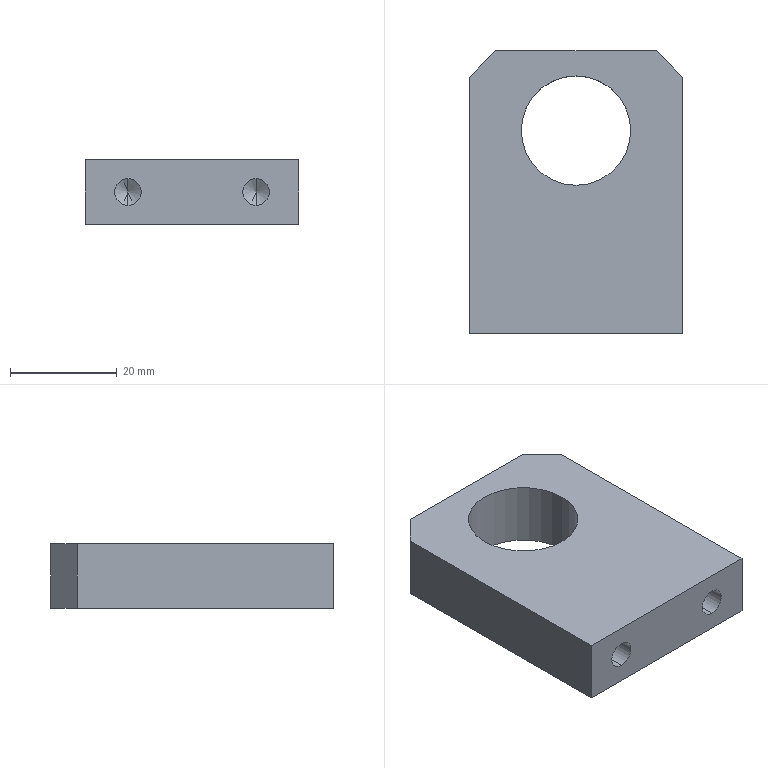Part | STEP file | 1 solid | 18 faces | box 40 x 53 x 12 mm | volume 20571 mm3 | plane 8 | cylinder 6 | cone 4 | commonest cylinder face diameters 5 x4 20.5 x2
STEP:
#1=CARTESIAN_POINT('',(0.,0.,0.));
#2=DIRECTION('',(0.,0.,1.));
#3=DIRECTION('',(1.,0.,0.));
#4=AXIS2_PLACEMENT_3D('',#1,#2,#3);
#5=CARTESIAN_POINT('',(8.,15.,3.5));
#6=VERTEX_POINT('',#5);
#7=CARTESIAN_POINT('',(8.,0.,3.5));
#8=VERTEX_POINT('',#7);
#9=CARTESIAN_POINT('',(8.,0.,3.5));
#10=DIRECTION('',(0.,-1.,0.));
#11=VECTOR('',#10,1.);
#12=LINE('',#9,#11);
#13=CARTESIAN_POINT('',(8.,0.,6.));
#14=DIRECTION('',(0.,-1.,0.));
#15=DIRECTION('',(0.,0.,-1.));
#16=AXIS2_PLACEMENT_3D('',#13,#14,#15);
#17=CYLINDRICAL_SURFACE('',#16,2.5);
#18=CARTESIAN_POINT('',(6.283,0.));
#19=DIRECTION('',(0.,1.));
#20=VECTOR('',#19,1.);
#21=LINE('',#18,#20);
#22=(GEOMETRIC_REPRESENTATION_CONTEXT(2)PARAMETRIC_REPRESENTATION_CONTEXT()REPRESENTATION_CONTEXT('',''));
#23=DEFINITIONAL_REPRESENTATION('',(#21),#22);
#24=PCURVE('',#17,#23);
#25=CARTESIAN_POINT('',(8.,0.,6.));
#26=DIRECTION('',(0.,-1.,0.));
#27=DIRECTION('',(0.,0.,-1.));
#28=AXIS2_PLACEMENT_3D('',#25,#26,#27);
#29=CYLINDRICAL_SURFACE('',#28,2.5);
#30=CARTESIAN_POINT('',(0.,0.));
#31=DIRECTION('',(0.,1.));
#32=VECTOR('',#31,1.);
#33=LINE('',#30,#32);
#34=(GEOMETRIC_REPRESENTATION_CONTEXT(2)PARAMETRIC_REPRESENTATION_CONTEXT()REPRESENTATION_CONTEXT('',''));
#35=DEFINITIONAL_REPRESENTATION('',(#33),#34);
#36=PCURVE('',#29,#35);
#37=SURFACE_CURVE('',#12,(#24,#36),.PCURVE_S1.);
#38=EDGE_CURVE('',#6,#8,#37,.T.);
#39=ORIENTED_EDGE('',*,*,#38,.T.);
#40=CARTESIAN_POINT('',(8.,0.,8.5));
#41=VERTEX_POINT('',#40);
#42=CARTESIAN_POINT('',(8.,0.,6.));
#43=DIRECTION('',(0.,-1.,0.));
#44=DIRECTION('',(0.,0.,-1.));
#45=AXIS2_PLACEMENT_3D('',#42,#43,#44);
#46=CIRCLE('',#45,2.5);
#47=CARTESIAN_POINT('',(0.,0.));
#48=DIRECTION('',(1.,0.));
#49=VECTOR('',#48,1.);
#50=LINE('',#47,#49);
#51=(GEOMETRIC_REPRESENTATION_CONTEXT(2)PARAMETRIC_REPRESENTATION_CONTEXT()REPRESENTATION_CONTEXT('',''));
#52=DEFINITIONAL_REPRESENTATION('',(#50),#51);
#53=PCURVE('',#17,#52);
#54=CARTESIAN_POINT('',(0.,0.,12.));
#55=DIRECTION('',(0.,1.,0.));
#56=DIRECTION('',(0.,0.,1.));
#57=AXIS2_PLACEMENT_3D('',#54,#55,#56);
#58=PLANE('',#57);
#59=CARTESIAN_POINT('',(-8.5,8.));
#60=CARTESIAN_POINT('',(-8.5,12.33));
#61=CARTESIAN_POINT('',(-4.75,10.165));
#62=CARTESIAN_POINT('',(-1.,8.));
#63=CARTESIAN_POINT('',(-4.75,5.835));
#64=CARTESIAN_POINT('',(-8.5,3.67));
#65=CARTESIAN_POINT('',(-8.5,8.));
#66=(BOUNDED_CURVE()B_SPLINE_CURVE(2,(#59,#60,#61,#62,#63,#64,#65),.UNSPECIFIED.,.T.,.F.)B_SPLINE_CURVE_WITH_KNOTS((1,2,2,2,2,1),(-2.094,0.,2.094,4.189,6.283,8.378),.UNSPECIFIED.)CURVE()GEOMETRIC_REPRESENTATION_ITEM()RATIONAL_B_SPLINE_CURVE((1.,0.5,1.,0.5,1.,0.5,1.))REPRESENTATION_ITEM(''));
#67=(GEOMETRIC_REPRESENTATION_CONTEXT(2)PARAMETRIC_REPRESENTATION_CONTEXT()REPRESENTATION_CONTEXT('',''));
#68=DEFINITIONAL_REPRESENTATION('',(#66),#67);
#69=PCURVE('',#58,#68);
#70=SURFACE_CURVE('',#46,(#53,#69),.PCURVE_S1.);
#71=EDGE_CURVE('',#41,#8,#70,.T.);
#72=ORIENTED_EDGE('',*,*,#71,.F.);
#73=CARTESIAN_POINT('',(8.,15.,8.5));
#74=VERTEX_POINT('',#73);
#75=CARTESIAN_POINT('',(8.,0.,8.5));
#76=DIRECTION('',(0.,-1.,0.));
#77=VECTOR('',#76,1.);
#78=LINE('',#75,#77);
#79=CARTESIAN_POINT('',(3.142,0.));
#80=DIRECTION('',(0.,1.));
#81=VECTOR('',#80,1.);
#82=LINE('',#79,#81);
#83=(GEOMETRIC_REPRESENTATION_CONTEXT(2)PARAMETRIC_REPRESENTATION_CONTEXT()REPRESENTATION_CONTEXT('',''));
#84=DEFINITIONAL_REPRESENTATION('',(#82),#83);
#85=PCURVE('',#17,#84);
#86=CARTESIAN_POINT('',(3.142,0.));
#87=DIRECTION('',(0.,1.));
#88=VECTOR('',#87,1.);
#89=LINE('',#86,#88);
#90=(GEOMETRIC_REPRESENTATION_CONTEXT(2)PARAMETRIC_REPRESENTATION_CONTEXT()REPRESENTATION_CONTEXT('',''));
#91=DEFINITIONAL_REPRESENTATION('',(#89),#90);
#92=PCURVE('',#29,#91);
#93=SURFACE_CURVE('',#78,(#85,#92),.PCURVE_S1.);
#94=EDGE_CURVE('',#74,#41,#93,.T.);
#95=ORIENTED_EDGE('',*,*,#94,.F.);
#96=CARTESIAN_POINT('',(8.,15.,6.));
#97=DIRECTION('',(0.,-1.,0.));
#98=DIRECTION('',(0.,0.,-1.));
#99=AXIS2_PLACEMENT_3D('',#96,#97,#98);
#100=CIRCLE('',#99,2.5);
#101=CARTESIAN_POINT('',(0.,-15.));
#102=DIRECTION('',(1.,0.));
#103=VECTOR('',#102,1.);
#104=LINE('',#101,#103);
#105=(GEOMETRIC_REPRESENTATION_CONTEXT(2)PARAMETRIC_REPRESENTATION_CONTEXT()REPRESENTATION_CONTEXT('',''));
#106=DEFINITIONAL_REPRESENTATION('',(#104),#105);
#107=PCURVE('',#17,#106);
#108=CARTESIAN_POINT('',(8.,15.,6.));
#109=DIRECTION('',(0.,-1.,0.));
#110=DIRECTION('',(0.,0.,-1.));
#111=AXIS2_PLACEMENT_3D('',#108,#109,#110);
#112=CONICAL_SURFACE('',#111,2.5,1.03);
#113=CARTESIAN_POINT('',(0.,0.));
#114=DIRECTION('',(1.,0.));
#115=VECTOR('',#114,1.);
#116=LINE('',#113,#115);
#117=(GEOMETRIC_REPRESENTATION_CONTEXT(2)PARAMETRIC_REPRESENTATION_CONTEXT()REPRESENTATION_CONTEXT('',''));
#118=DEFINITIONAL_REPRESENTATION('',(#116),#117);
#119=PCURVE('',#112,#118);
#120=SURFACE_CURVE('',#100,(#107,#119),.PCURVE_S1.);
#121=EDGE_CURVE('',#74,#6,#120,.T.);
#122=ORIENTED_EDGE('',*,*,#121,.T.);
#123=EDGE_LOOP('',(#39,#72,#95,#122));
#124=FACE_BOUND('',#123,.F.);
#125=ADVANCED_FACE('',(#124),#17,.F.);
#126=ORIENTED_EDGE('',*,*,#121,.F.);
#127=CARTESIAN_POINT('',(8.,16.502,6.));
#128=VERTEX_POINT('',#127);
#129=CARTESIAN_POINT('',(8.,15.,8.5));
#130=DIRECTION('',(0.,-0.515,0.8572));
#131=VECTOR('',#130,1.);
#132=LINE('',#129,#131);
#133=CARTESIAN_POINT('',(3.142,0.));
#134=DIRECTION('',(0.,1.));
#135=VECTOR('',#134,1.);
#136=LINE('',#133,#135);
#137=(GEOMETRIC_REPRESENTATION_CONTEXT(2)PARAMETRIC_REPRESENTATION_CONTEXT()REPRESENTATION_CONTEXT('',''));
#138=DEFINITIONAL_REPRESENTATION('',(#136),#137);
#139=PCURVE('',#112,#138);
#140=CARTESIAN_POINT('',(8.,15.,6.));
#141=DIRECTION('',(0.,-1.,0.));
#142=DIRECTION('',(0.,0.,-1.));
#143=AXIS2_PLACEMENT_3D('',#140,#141,#142);
#144=CONICAL_SURFACE('',#143,2.5,1.03);
#145=CARTESIAN_POINT('',(3.142,0.));
#146=DIRECTION('',(0.,1.));
#147=VECTOR('',#146,1.);
#148=LINE('',#145,#147);
#149=(GEOMETRIC_REPRESENTATION_CONTEXT(2)PARAMETRIC_REPRESENTATION_CONTEXT()REPRESENTATION_CONTEXT('',''));
#150=DEFINITIONAL_REPRESENTATION('',(#148),#149);
#151=PCURVE('',#144,#150);
#152=SURFACE_CURVE('',#132,(#139,#151),.PCURVE_S1.);
#153=EDGE_CURVE('',#128,#74,#152,.T.);
#154=ORIENTED_EDGE('',*,*,#153,.F.);
#155=CARTESIAN_POINT('',(8.,15.,3.5));
#156=DIRECTION('',(0.,-0.515,-0.8572));
#157=VECTOR('',#156,1.);
#158=LINE('',#155,#157);
#159=CARTESIAN_POINT('',(6.283,0.));
#160=DIRECTION('',(0.,1.));
#161=VECTOR('',#160,1.);
#162=LINE('',#159,#161);
#163=(GEOMETRIC_REPRESENTATION_CONTEXT(2)PARAMETRIC_REPRESENTATION_CONTEXT()REPRESENTATION_CONTEXT('',''));
#164=DEFINITIONAL_REPRESENTATION('',(#162),#163);
#165=PCURVE('',#112,#164);
#166=CARTESIAN_POINT('',(0.,0.));
#167=DIRECTION('',(0.,1.));
#168=VECTOR('',#167,1.);
#169=LINE('',#166,#168);
#170=(GEOMETRIC_REPRESENTATION_CONTEXT(2)PARAMETRIC_REPRESENTATION_CONTEXT()REPRESENTATION_CONTEXT('',''));
#171=DEFINITIONAL_REPRESENTATION('',(#169),#170);
#172=PCURVE('',#144,#171);
#173=SURFACE_CURVE('',#158,(#165,#172),.PCURVE_S1.);
#174=EDGE_CURVE('',#128,#6,#173,.T.);
#175=ORIENTED_EDGE('',*,*,#174,.T.);
#176=EDGE_LOOP('',(#126,#154,#175));
#177=FACE_BOUND('',#176,.F.);
#178=ADVANCED_FACE('',(#177),#112,.F.);
#179=CARTESIAN_POINT('',(32.,15.,3.5));
#180=VERTEX_POINT('',#179);
#181=CARTESIAN_POINT('',(32.,0.,3.5));
#182=VERTEX_POINT('',#181);
#183=CARTESIAN_POINT('',(32.,0.,3.5));
#184=DIRECTION('',(0.,-1.,0.));
#185=VECTOR('',#184,1.);
#186=LINE('',#183,#185);
#187=CARTESIAN_POINT('',(32.,0.,6.));
#188=DIRECTION('',(0.,-1.,0.));
#189=DIRECTION('',(0.,0.,-1.));
#190=AXIS2_PLACEMENT_3D('',#187,#188,#189);
#191=CYLINDRICAL_SURFACE('',#190,2.5);
#192=CARTESIAN_POINT('',(6.283,0.));
#193=DIRECTION('',(0.,1.));
#194=VECTOR('',#193,1.);
#195=LINE('',#192,#194);
#196=(GEOMETRIC_REPRESENTATION_CONTEXT(2)PARAMETRIC_REPRESENTATION_CONTEXT()REPRESENTATION_CONTEXT('',''));
#197=DEFINITIONAL_REPRESENTATION('',(#195),#196);
#198=PCURVE('',#191,#197);
#199=CARTESIAN_POINT('',(32.,0.,6.));
#200=DIRECTION('',(0.,-1.,0.));
#201=DIRECTION('',(0.,0.,-1.));
#202=AXIS2_PLACEMENT_3D('',#199,#200,#201);
#203=CYLINDRICAL_SURFACE('',#202,2.5);
#204=CARTESIAN_POINT('',(0.,0.));
#205=DIRECTION('',(0.,1.));
#206=VECTOR('',#205,1.);
#207=LINE('',#204,#206);
#208=(GEOMETRIC_REPRESENTATION_CONTEXT(2)PARAMETRIC_REPRESENTATION_CONTEXT()REPRESENTATION_CONTEXT('',''));
#209=DEFINITIONAL_REPRESENTATION('',(#207),#208);
#210=PCURVE('',#203,#209);
#211=SURFACE_CURVE('',#186,(#198,#210),.PCURVE_S1.);
#212=EDGE_CURVE('',#180,#182,#211,.T.);
#213=ORIENTED_EDGE('',*,*,#212,.T.);
#214=CARTESIAN_POINT('',(32.,0.,8.5));
#215=VERTEX_POINT('',#214);
#216=CARTESIAN_POINT('',(32.,0.,6.));
#217=DIRECTION('',(0.,-1.,0.));
#218=DIRECTION('',(0.,0.,-1.));
#219=AXIS2_PLACEMENT_3D('',#216,#217,#218);
#220=CIRCLE('',#219,2.5);
#221=CARTESIAN_POINT('',(0.,0.));
#222=DIRECTION('',(1.,0.));
#223=VECTOR('',#222,1.);
#224=LINE('',#221,#223);
#225=(GEOMETRIC_REPRESENTATION_CONTEXT(2)PARAMETRIC_REPRESENTATION_CONTEXT()REPRESENTATION_CONTEXT('',''));
#226=DEFINITIONAL_REPRESENTATION('',(#224),#225);
#227=PCURVE('',#191,#226);
#228=CARTESIAN_POINT('',(-8.5,32.));
#229=CARTESIAN_POINT('',(-8.5,36.33));
#230=CARTESIAN_POINT('',(-4.75,34.165));
#231=CARTESIAN_POINT('',(-1.,32.));
#232=CARTESIAN_POINT('',(-4.75,29.835));
#233=CARTESIAN_POINT('',(-8.5,27.67));
#234=CARTESIAN_POINT('',(-8.5,32.));
#235=(BOUNDED_CURVE()B_SPLINE_CURVE(2,(#228,#229,#230,#231,#232,#233,#234),.UNSPECIFIED.,.T.,.F.)B_SPLINE_CURVE_WITH_KNOTS((1,2,2,2,2,1),(-2.094,0.,2.094,4.189,6.283,8.378),.UNSPECIFIED.)CURVE()GEOMETRIC_REPRESENTATION_ITEM()RATIONAL_B_SPLINE_CURVE((1.,0.5,1.,0.5,1.,0.5,1.))REPRESENTATION_ITEM(''));
#236=(GEOMETRIC_REPRESENTATION_CONTEXT(2)PARAMETRIC_REPRESENTATION_CONTEXT()REPRESENTATION_CONTEXT('',''));
#237=DEFINITIONAL_REPRESENTATION('',(#235),#236);
#238=PCURVE('',#58,#237);
#239=SURFACE_CURVE('',#220,(#227,#238),.PCURVE_S1.);
#240=EDGE_CURVE('',#215,#182,#239,.T.);
#241=ORIENTED_EDGE('',*,*,#240,.F.);
#242=CARTESIAN_POINT('',(32.,15.,8.5));
#243=VERTEX_POINT('',#242);
#244=CARTESIAN_POINT('',(32.,0.,8.5));
#245=DIRECTION('',(0.,-1.,0.));
#246=VECTOR('',#245,1.);
#247=LINE('',#244,#246);
#248=CARTESIAN_POINT('',(3.142,0.));
#249=DIRECTION('',(0.,1.));
#250=VECTOR('',#249,1.);
#251=LINE('',#248,#250);
#252=(GEOMETRIC_REPRESENTATION_CONTEXT(2)PARAMETRIC_REPRESENTATION_CONTEXT()REPRESENTATION_CONTEXT('',''));
#253=DEFINITIONAL_REPRESENTATION('',(#251),#252);
#254=PCURVE('',#191,#253);
#255=CARTESIAN_POINT('',(3.142,0.));
#256=DIRECTION('',(0.,1.));
#257=VECTOR('',#256,1.);
#258=LINE('',#255,#257);
#259=(GEOMETRIC_REPRESENTATION_CONTEXT(2)PARAMETRIC_REPRESENTATION_CONTEXT()REPRESENTATION_CONTEXT('',''));
#260=DEFINITIONAL_REPRESENTATION('',(#258),#259);
#261=PCURVE('',#203,#260);
#262=SURFACE_CURVE('',#247,(#254,#261),.PCURVE_S1.);
#263=EDGE_CURVE('',#243,#215,#262,.T.);
#264=ORIENTED_EDGE('',*,*,#263,.F.);
#265=CARTESIAN_POINT('',(32.,15.,6.));
#266=DIRECTION('',(0.,-1.,0.));
#267=DIRECTION('',(0.,0.,-1.));
#268=AXIS2_PLACEMENT_3D('',#265,#266,#267);
#269=CIRCLE('',#268,2.5);
#270=CARTESIAN_POINT('',(0.,-15.));
#271=DIRECTION('',(1.,0.));
#272=VECTOR('',#271,1.);
#273=LINE('',#270,#272);
#274=(GEOMETRIC_REPRESENTATION_CONTEXT(2)PARAMETRIC_REPRESENTATION_CONTEXT()REPRESENTATION_CONTEXT('',''));
#275=DEFINITIONAL_REPRESENTATION('',(#273),#274);
#276=PCURVE('',#191,#275);
#277=CARTESIAN_POINT('',(32.,15.,6.));
#278=DIRECTION('',(0.,-1.,0.));
#279=DIRECTION('',(0.,0.,-1.));
#280=AXIS2_PLACEMENT_3D('',#277,#278,#279);
#281=CONICAL_SURFACE('',#280,2.5,1.03);
#282=CARTESIAN_POINT('',(0.,0.));
#283=DIRECTION('',(1.,0.));
#284=VECTOR('',#283,1.);
#285=LINE('',#282,#284);
#286=(GEOMETRIC_REPRESENTATION_CONTEXT(2)PARAMETRIC_REPRESENTATION_CONTEXT()REPRESENTATION_CONTEXT('',''));
#287=DEFINITIONAL_REPRESENTATION('',(#285),#286);
#288=PCURVE('',#281,#287);
#289=SURFACE_CURVE('',#269,(#276,#288),.PCURVE_S1.);
#290=EDGE_CURVE('',#243,#180,#289,.T.);
#291=ORIENTED_EDGE('',*,*,#290,.T.);
#292=EDGE_LOOP('',(#213,#241,#264,#291));
#293=FACE_BOUND('',#292,.F.);
#294=ADVANCED_FACE('',(#293),#191,.F.);
#295=ORIENTED_EDGE('',*,*,#290,.F.);
#296=CARTESIAN_POINT('',(32.,16.502,6.));
#297=VERTEX_POINT('',#296);
#298=CARTESIAN_POINT('',(32.,15.,8.5));
#299=DIRECTION('',(0.,-0.515,0.8572));
#300=VECTOR('',#299,1.);
#301=LINE('',#298,#300);
#302=CARTESIAN_POINT('',(3.142,0.));
#303=DIRECTION('',(0.,1.));
#304=VECTOR('',#303,1.);
#305=LINE('',#302,#304);
#306=(GEOMETRIC_REPRESENTATION_CONTEXT(2)PARAMETRIC_REPRESENTATION_CONTEXT()REPRESENTATION_CONTEXT('',''));
#307=DEFINITIONAL_REPRESENTATION('',(#305),#306);
#308=PCURVE('',#281,#307);
#309=CARTESIAN_POINT('',(32.,15.,6.));
#310=DIRECTION('',(0.,-1.,0.));
#311=DIRECTION('',(0.,0.,-1.));
#312=AXIS2_PLACEMENT_3D('',#309,#310,#311);
#313=CONICAL_SURFACE('',#312,2.5,1.03);
#314=CARTESIAN_POINT('',(3.142,0.));
#315=DIRECTION('',(0.,1.));
#316=VECTOR('',#315,1.);
#317=LINE('',#314,#316);
#318=(GEOMETRIC_REPRESENTATION_CONTEXT(2)PARAMETRIC_REPRESENTATION_CONTEXT()REPRESENTATION_CONTEXT('',''));
#319=DEFINITIONAL_REPRESENTATION('',(#317),#318);
#320=PCURVE('',#313,#319);
#321=SURFACE_CURVE('',#301,(#308,#320),.PCURVE_S1.);
#322=EDGE_CURVE('',#297,#243,#321,.T.);
#323=ORIENTED_EDGE('',*,*,#322,.F.);
#324=CARTESIAN_POINT('',(32.,15.,3.5));
#325=DIRECTION('',(0.,-0.515,-0.8572));
#326=VECTOR('',#325,1.);
#327=LINE('',#324,#326);
#328=CARTESIAN_POINT('',(6.283,0.));
#329=DIRECTION('',(0.,1.));
#330=VECTOR('',#329,1.);
#331=LINE('',#328,#330);
#332=(GEOMETRIC_REPRESENTATION_CONTEXT(2)PARAMETRIC_REPRESENTATION_CONTEXT()REPRESENTATION_CONTEXT('',''));
#333=DEFINITIONAL_REPRESENTATION('',(#331),#332);
#334=PCURVE('',#281,#333);
#335=CARTESIAN_POINT('',(0.,0.));
#336=DIRECTION('',(0.,1.));
#337=VECTOR('',#336,1.);
#338=LINE('',#335,#337);
#339=(GEOMETRIC_REPRESENTATION_CONTEXT(2)PARAMETRIC_REPRESENTATION_CONTEXT()REPRESENTATION_CONTEXT('',''));
#340=DEFINITIONAL_REPRESENTATION('',(#338),#339);
#341=PCURVE('',#313,#340);
#342=SURFACE_CURVE('',#327,(#334,#341),.PCURVE_S1.);
#343=EDGE_CURVE('',#297,#180,#342,.T.);
#344=ORIENTED_EDGE('',*,*,#343,.T.);
#345=EDGE_LOOP('',(#295,#323,#344));
#346=FACE_BOUND('',#345,.F.);
#347=ADVANCED_FACE('',(#346),#281,.F.);
#348=CARTESIAN_POINT('',(30.25,38.,0.));
#349=VERTEX_POINT('',#348);
#350=CARTESIAN_POINT('',(30.25,38.,12.));
#351=VERTEX_POINT('',#350);
#352=CARTESIAN_POINT('',(30.25,38.,0.));
#353=DIRECTION('',(0.,0.,1.));
#354=VECTOR('',#353,1.);
#355=LINE('',#352,#354);
#356=CARTESIAN_POINT('',(20.,38.,0.));
#357=DIRECTION('',(0.,0.,1.));
#358=DIRECTION('',(1.,0.,0.));
#359=AXIS2_PLACEMENT_3D('',#356,#357,#358);
#360=CYLINDRICAL_SURFACE('',#359,10.25);
#361=CARTESIAN_POINT('',(6.283,0.));
#362=DIRECTION('',(0.,1.));
#363=VECTOR('',#362,1.);
#364=LINE('',#361,#363);
#365=(GEOMETRIC_REPRESENTATION_CONTEXT(2)PARAMETRIC_REPRESENTATION_CONTEXT()REPRESENTATION_CONTEXT('',''));
#366=DEFINITIONAL_REPRESENTATION('',(#364),#365);
#367=PCURVE('',#360,#366);
#368=CARTESIAN_POINT('',(20.,38.,0.));
#369=DIRECTION('',(0.,0.,1.));
#370=DIRECTION('',(1.,0.,0.));
#371=AXIS2_PLACEMENT_3D('',#368,#369,#370);
#372=CYLINDRICAL_SURFACE('',#371,10.25);
#373=CARTESIAN_POINT('',(0.,0.));
#374=DIRECTION('',(0.,1.));
#375=VECTOR('',#374,1.);
#376=LINE('',#373,#375);
#377=(GEOMETRIC_REPRESENTATION_CONTEXT(2)PARAMETRIC_REPRESENTATION_CONTEXT()REPRESENTATION_CONTEXT('',''));
#378=DEFINITIONAL_REPRESENTATION('',(#376),#377);
#379=PCURVE('',#372,#378);
#380=SURFACE_CURVE('',#355,(#367,#379),.PCURVE_S1.);
#381=EDGE_CURVE('',#349,#351,#380,.T.);
#382=ORIENTED_EDGE('',*,*,#381,.T.);
#383=CARTESIAN_POINT('',(9.75,38.,12.));
#384=VERTEX_POINT('',#383);
#385=CARTESIAN_POINT('',(20.,38.,12.));
#386=DIRECTION('',(0.,0.,1.));
#387=DIRECTION('',(1.,0.,0.));
#388=AXIS2_PLACEMENT_3D('',#385,#386,#387);
#389=CIRCLE('',#388,10.25);
#390=CARTESIAN_POINT('',(0.,12.));
#391=DIRECTION('',(1.,0.));
#392=VECTOR('',#391,1.);
#393=LINE('',#390,#392);
#394=(GEOMETRIC_REPRESENTATION_CONTEXT(2)PARAMETRIC_REPRESENTATION_CONTEXT()REPRESENTATION_CONTEXT('',''));
#395=DEFINITIONAL_REPRESENTATION('',(#393),#394);
#396=PCURVE('',#360,#395);
#397=CARTESIAN_POINT('',(0.,0.,12.));
#398=DIRECTION('',(0.,0.,-1.));
#399=DIRECTION('',(-1.,0.,0.));
#400=AXIS2_PLACEMENT_3D('',#397,#398,#399);
#401=PLANE('',#400);
#402=CARTESIAN_POINT('',(-30.25,38.));
#403=CARTESIAN_POINT('',(-30.25,55.754));
#404=CARTESIAN_POINT('',(-14.875,46.877));
#405=CARTESIAN_POINT('',(0.5,38.));
#406=CARTESIAN_POINT('',(-14.875,29.123));
#407=CARTESIAN_POINT('',(-30.25,20.246));
#408=CARTESIAN_POINT('',(-30.25,38.));
#409=(BOUNDED_CURVE()B_SPLINE_CURVE(2,(#402,#403,#404,#405,#406,#407,#408),.UNSPECIFIED.,.T.,.F.)B_SPLINE_CURVE_WITH_KNOTS((1,2,2,2,2,1),(-2.094,0.,2.094,4.189,6.283,8.378),.UNSPECIFIED.)CURVE()GEOMETRIC_REPRESENTATION_ITEM()RATIONAL_B_SPLINE_CURVE((1.,0.5,1.,0.5,1.,0.5,1.))REPRESENTATION_ITEM(''));
#410=(GEOMETRIC_REPRESENTATION_CONTEXT(2)PARAMETRIC_REPRESENTATION_CONTEXT()REPRESENTATION_CONTEXT('',''));
#411=DEFINITIONAL_REPRESENTATION('',(#409),#410);
#412=PCURVE('',#401,#411);
#413=SURFACE_CURVE('',#389,(#396,#412),.PCURVE_S1.);
#414=EDGE_CURVE('',#384,#351,#413,.T.);
#415=ORIENTED_EDGE('',*,*,#414,.F.);
#416=CARTESIAN_POINT('',(9.75,38.,0.));
#417=VERTEX_POINT('',#416);
#418=CARTESIAN_POINT('',(9.75,38.,0.));
#419=DIRECTION('',(0.,0.,1.));
#420=VECTOR('',#419,1.);
#421=LINE('',#418,#420);
#422=CARTESIAN_POINT('',(3.142,0.));
#423=DIRECTION('',(0.,1.));
#424=VECTOR('',#423,1.);
#425=LINE('',#422,#424);
#426=(GEOMETRIC_REPRESENTATION_CONTEXT(2)PARAMETRIC_REPRESENTATION_CONTEXT()REPRESENTATION_CONTEXT('',''));
#427=DEFINITIONAL_REPRESENTATION('',(#425),#426);
#428=PCURVE('',#360,#427);
#429=CARTESIAN_POINT('',(3.142,0.));
#430=DIRECTION('',(0.,1.));
#431=VECTOR('',#430,1.);
#432=LINE('',#429,#431);
#433=(GEOMETRIC_REPRESENTATION_CONTEXT(2)PARAMETRIC_REPRESENTATION_CONTEXT()REPRESENTATION_CONTEXT('',''));
#434=DEFINITIONAL_REPRESENTATION('',(#432),#433);
#435=PCURVE('',#372,#434);
#436=SURFACE_CURVE('',#421,(#428,#435),.PCURVE_S1.);
#437=EDGE_CURVE('',#417,#384,#436,.T.);
#438=ORIENTED_EDGE('',*,*,#437,.F.);
#439=CARTESIAN_POINT('',(20.,38.,0.));
#440=DIRECTION('',(0.,0.,1.));
#441=DIRECTION('',(1.,0.,0.));
#442=AXIS2_PLACEMENT_3D('',#439,#440,#441);
#443=CIRCLE('',#442,10.25);
#444=CARTESIAN_POINT('',(0.,0.));
#445=DIRECTION('',(1.,0.));
#446=VECTOR('',#445,1.);
#447=LINE('',#444,#446);
#448=(GEOMETRIC_REPRESENTATION_CONTEXT(2)PARAMETRIC_REPRESENTATION_CONTEXT()REPRESENTATION_CONTEXT('',''));
#449=DEFINITIONAL_REPRESENTATION('',(#447),#448);
#450=PCURVE('',#360,#449);
#451=CARTESIAN_POINT('',(0.,0.,0.));
#452=DIRECTION('',(0.,0.,-1.));
#453=DIRECTION('',(-1.,0.,0.));
#454=AXIS2_PLACEMENT_3D('',#451,#452,#453);
#455=PLANE('',#454);
#456=CARTESIAN_POINT('',(-30.25,38.));
#457=CARTESIAN_POINT('',(-30.25,55.754));
#458=CARTESIAN_POINT('',(-14.875,46.877));
#459=CARTESIAN_POINT('',(0.5,38.));
#460=CARTESIAN_POINT('',(-14.875,29.123));
#461=CARTESIAN_POINT('',(-30.25,20.246));
#462=CARTESIAN_POINT('',(-30.25,38.));
#463=(BOUNDED_CURVE()B_SPLINE_CURVE(2,(#456,#457,#458,#459,#460,#461,#462),.UNSPECIFIED.,.T.,.F.)B_SPLINE_CURVE_WITH_KNOTS((1,2,2,2,2,1),(-2.094,0.,2.094,4.189,6.283,8.378),.UNSPECIFIED.)CURVE()GEOMETRIC_REPRESENTATION_ITEM()RATIONAL_B_SPLINE_CURVE((1.,0.5,1.,0.5,1.,0.5,1.))REPRESENTATION_ITEM(''));
#464=(GEOMETRIC_REPRESENTATION_CONTEXT(2)PARAMETRIC_REPRESENTATION_CONTEXT()REPRESENTATION_CONTEXT('',''));
#465=DEFINITIONAL_REPRESENTATION('',(#463),#464);
#466=PCURVE('',#455,#465);
#467=SURFACE_CURVE('',#443,(#450,#466),.PCURVE_S1.);
#468=EDGE_CURVE('',#417,#349,#467,.T.);
#469=ORIENTED_EDGE('',*,*,#468,.T.);
#470=EDGE_LOOP('',(#382,#415,#438,#469));
#471=FACE_BOUND('',#470,.F.);
#472=ADVANCED_FACE('',(#471),#360,.F.);
#473=CARTESIAN_POINT('',(0.,48.,12.));
#474=VERTEX_POINT('',#473);
#475=CARTESIAN_POINT('',(0.,0.,12.));
#476=VERTEX_POINT('',#475);
#477=CARTESIAN_POINT('',(0.,0.,12.));
#478=DIRECTION('',(0.,-1.,0.));
#479=VECTOR('',#478,1.);
#480=LINE('',#477,#479);
#481=CARTESIAN_POINT('',(0.,0.,12.));
#482=DIRECTION('',(1.,0.,0.));
#483=DIRECTION('',(0.,0.,-1.));
#484=AXIS2_PLACEMENT_3D('',#481,#482,#483);
#485=PLANE('',#484);
#486=CARTESIAN_POINT('',(0.,0.));
#487=DIRECTION('',(0.,-1.));
#488=VECTOR('',#487,1.);
#489=LINE('',#486,#488);
#490=(GEOMETRIC_REPRESENTATION_CONTEXT(2)PARAMETRIC_REPRESENTATION_CONTEXT()REPRESENTATION_CONTEXT('',''));
#491=DEFINITIONAL_REPRESENTATION('',(#489),#490);
#492=PCURVE('',#485,#491);
#493=CARTESIAN_POINT('',(0.,0.));
#494=DIRECTION('',(0.,-1.));
#495=VECTOR('',#494,1.);
#496=LINE('',#493,#495);
#497=(GEOMETRIC_REPRESENTATION_CONTEXT(2)PARAMETRIC_REPRESENTATION_CONTEXT()REPRESENTATION_CONTEXT('',''));
#498=DEFINITIONAL_REPRESENTATION('',(#496),#497);
#499=PCURVE('',#401,#498);
#500=SURFACE_CURVE('',#480,(#492,#499),.PCURVE_S1.);
#501=EDGE_CURVE('',#474,#476,#500,.T.);
#502=ORIENTED_EDGE('',*,*,#501,.F.);
#503=CARTESIAN_POINT('',(0.,48.,0.));
#504=VERTEX_POINT('',#503);
#505=CARTESIAN_POINT('',(0.,48.,12.));
#506=DIRECTION('',(0.,0.,-1.));
#507=VECTOR('',#506,1.);
#508=LINE('',#505,#507);
#509=CARTESIAN_POINT('',(0.,48.));
#510=DIRECTION('',(1.,0.));
#511=VECTOR('',#510,1.);
#512=LINE('',#509,#511);
#513=(GEOMETRIC_REPRESENTATION_CONTEXT(2)PARAMETRIC_REPRESENTATION_CONTEXT()REPRESENTATION_CONTEXT('',''));
#514=DEFINITIONAL_REPRESENTATION('',(#512),#513);
#515=PCURVE('',#485,#514);
#516=CARTESIAN_POINT('',(0.,48.,12.));
#517=DIRECTION('',(0.7071,-0.7071,0.));
#518=DIRECTION('',(0.,0.,-1.));
#519=AXIS2_PLACEMENT_3D('',#516,#517,#518);
#520=PLANE('',#519);
#521=CARTESIAN_POINT('',(0.,0.));
#522=DIRECTION('',(1.,0.));
#523=VECTOR('',#522,1.);
#524=LINE('',#521,#523);
#525=(GEOMETRIC_REPRESENTATION_CONTEXT(2)PARAMETRIC_REPRESENTATION_CONTEXT()REPRESENTATION_CONTEXT('',''));
#526=DEFINITIONAL_REPRESENTATION('',(#524),#525);
#527=PCURVE('',#520,#526);
#528=SURFACE_CURVE('',#508,(#515,#527),.PCURVE_S1.);
#529=EDGE_CURVE('',#474,#504,#528,.T.);
#530=ORIENTED_EDGE('',*,*,#529,.T.);
#531=CARTESIAN_POINT('',(0.,0.,0.));
#532=VERTEX_POINT('',#531);
#533=CARTESIAN_POINT('',(0.,0.,0.));
#534=DIRECTION('',(0.,-1.,0.));
#535=VECTOR('',#534,1.);
#536=LINE('',#533,#535);
#537=CARTESIAN_POINT('',(12.,0.));
#538=DIRECTION('',(0.,-1.));
#539=VECTOR('',#538,1.);
#540=LINE('',#537,#539);
#541=(GEOMETRIC_REPRESENTATION_CONTEXT(2)PARAMETRIC_REPRESENTATION_CONTEXT()REPRESENTATION_CONTEXT('',''));
#542=DEFINITIONAL_REPRESENTATION('',(#540),#541);
#543=PCURVE('',#485,#542);
#544=CARTESIAN_POINT('',(0.,0.));
#545=DIRECTION('',(0.,-1.));
#546=VECTOR('',#545,1.);
#547=LINE('',#544,#546);
#548=(GEOMETRIC_REPRESENTATION_CONTEXT(2)PARAMETRIC_REPRESENTATION_CONTEXT()REPRESENTATION_CONTEXT('',''));
#549=DEFINITIONAL_REPRESENTATION('',(#547),#548);
#550=PCURVE('',#455,#549);
#551=SURFACE_CURVE('',#536,(#543,#550),.PCURVE_S1.);
#552=EDGE_CURVE('',#504,#532,#551,.T.);
#553=ORIENTED_EDGE('',*,*,#552,.T.);
#554=CARTESIAN_POINT('',(0.,0.,12.));
#555=DIRECTION('',(0.,0.,-1.));
#556=VECTOR('',#555,1.);
#557=LINE('',#554,#556);
#558=CARTESIAN_POINT('',(0.,0.));
#559=DIRECTION('',(1.,0.));
#560=VECTOR('',#559,1.);
#561=LINE('',#558,#560);
#562=(GEOMETRIC_REPRESENTATION_CONTEXT(2)PARAMETRIC_REPRESENTATION_CONTEXT()REPRESENTATION_CONTEXT('',''));
#563=DEFINITIONAL_REPRESENTATION('',(#561),#562);
#564=PCURVE('',#485,#563);
#565=CARTESIAN_POINT('',(0.,0.));
#566=DIRECTION('',(-1.,0.));
#567=VECTOR('',#566,1.);
#568=LINE('',#565,#567);
#569=(GEOMETRIC_REPRESENTATION_CONTEXT(2)PARAMETRIC_REPRESENTATION_CONTEXT()REPRESENTATION_CONTEXT('',''));
#570=DEFINITIONAL_REPRESENTATION('',(#568),#569);
#571=PCURVE('',#58,#570);
#572=SURFACE_CURVE('',#557,(#564,#571),.PCURVE_S1.);
#573=EDGE_CURVE('',#476,#532,#572,.T.);
#574=ORIENTED_EDGE('',*,*,#573,.F.);
#575=EDGE_LOOP('',(#502,#530,#553,#574));
#576=FACE_BOUND('',#575,.T.);
#577=ADVANCED_FACE('',(#576),#485,.F.);
#578=CARTESIAN_POINT('',(8.,0.,6.));
#579=DIRECTION('',(0.,-1.,0.));
#580=DIRECTION('',(0.,0.,-1.));
#581=AXIS2_PLACEMENT_3D('',#578,#579,#580);
#582=CIRCLE('',#581,2.5);
#583=CARTESIAN_POINT('',(-8.5,8.));
#584=CARTESIAN_POINT('',(-8.5,12.33));
#585=CARTESIAN_POINT('',(-4.75,10.165));
#586=CARTESIAN_POINT('',(-1.,8.));
#587=CARTESIAN_POINT('',(-4.75,5.835));
#588=CARTESIAN_POINT('',(-8.5,3.67));
#589=CARTESIAN_POINT('',(-8.5,8.));
#590=(BOUNDED_CURVE()B_SPLINE_CURVE(2,(#583,#584,#585,#586,#587,#588,#589),.UNSPECIFIED.,.T.,.F.)B_SPLINE_CURVE_WITH_KNOTS((1,2,2,2,2,1),(-2.094,0.,2.094,4.189,6.283,8.378),.UNSPECIFIED.)CURVE()GEOMETRIC_REPRESENTATION_ITEM()RATIONAL_B_SPLINE_CURVE((1.,0.5,1.,0.5,1.,0.5,1.))REPRESENTATION_ITEM(''));
#591=(GEOMETRIC_REPRESENTATION_CONTEXT(2)PARAMETRIC_REPRESENTATION_CONTEXT()REPRESENTATION_CONTEXT('',''));
#592=DEFINITIONAL_REPRESENTATION('',(#590),#591);
#593=PCURVE('',#58,#592);
#594=CARTESIAN_POINT('',(0.,0.));
#595=DIRECTION('',(1.,0.));
#596=VECTOR('',#595,1.);
#597=LINE('',#594,#596);
#598=(GEOMETRIC_REPRESENTATION_CONTEXT(2)PARAMETRIC_REPRESENTATION_CONTEXT()REPRESENTATION_CONTEXT('',''));
#599=DEFINITIONAL_REPRESENTATION('',(#597),#598);
#600=PCURVE('',#29,#599);
#601=SURFACE_CURVE('',#582,(#593,#600),.PCURVE_S1.);
#602=EDGE_CURVE('',#8,#41,#601,.T.);
#603=ORIENTED_EDGE('',*,*,#602,.F.);
#604=ORIENTED_EDGE('',*,*,#71,.F.);
#605=EDGE_LOOP('',(#603,#604));
#606=FACE_BOUND('',#605,.T.);
#607=CARTESIAN_POINT('',(32.,0.,6.));
#608=DIRECTION('',(0.,-1.,0.));
#609=DIRECTION('',(0.,0.,-1.));
#610=AXIS2_PLACEMENT_3D('',#607,#608,#609);
#611=CIRCLE('',#610,2.5);
#612=CARTESIAN_POINT('',(-8.5,32.));
#613=CARTESIAN_POINT('',(-8.5,36.33));
#614=CARTESIAN_POINT('',(-4.75,34.165));
#615=CARTESIAN_POINT('',(-1.,32.));
#616=CARTESIAN_POINT('',(-4.75,29.835));
#617=CARTESIAN_POINT('',(-8.5,27.67));
#618=CARTESIAN_POINT('',(-8.5,32.));
#619=(BOUNDED_CURVE()B_SPLINE_CURVE(2,(#612,#613,#614,#615,#616,#617,#618),.UNSPECIFIED.,.T.,.F.)B_SPLINE_CURVE_WITH_KNOTS((1,2,2,2,2,1),(-2.094,0.,2.094,4.189,6.283,8.378),.UNSPECIFIED.)CURVE()GEOMETRIC_REPRESENTATION_ITEM()RATIONAL_B_SPLINE_CURVE((1.,0.5,1.,0.5,1.,0.5,1.))REPRESENTATION_ITEM(''));
#620=(GEOMETRIC_REPRESENTATION_CONTEXT(2)PARAMETRIC_REPRESENTATION_CONTEXT()REPRESENTATION_CONTEXT('',''));
#621=DEFINITIONAL_REPRESENTATION('',(#619),#620);
#622=PCURVE('',#58,#621);
#623=CARTESIAN_POINT('',(0.,0.));
#624=DIRECTION('',(1.,0.));
#625=VECTOR('',#624,1.);
#626=LINE('',#623,#625);
#627=(GEOMETRIC_REPRESENTATION_CONTEXT(2)PARAMETRIC_REPRESENTATION_CONTEXT()REPRESENTATION_CONTEXT('',''));
#628=DEFINITIONAL_REPRESENTATION('',(#626),#627);
#629=PCURVE('',#203,#628);
#630=SURFACE_CURVE('',#611,(#622,#629),.PCURVE_S1.);
#631=EDGE_CURVE('',#182,#215,#630,.T.);
#632=ORIENTED_EDGE('',*,*,#631,.F.);
#633=ORIENTED_EDGE('',*,*,#240,.F.);
#634=EDGE_LOOP('',(#632,#633));
#635=FACE_BOUND('',#634,.T.);
#636=CARTESIAN_POINT('',(40.,0.,0.));
#637=VERTEX_POINT('',#636);
#638=CARTESIAN_POINT('',(0.,0.,0.));
#639=DIRECTION('',(1.,0.,0.));
#640=VECTOR('',#639,1.);
#641=LINE('',#638,#640);
#642=CARTESIAN_POINT('',(-12.,0.));
#643=DIRECTION('',(0.,1.));
#644=VECTOR('',#643,1.);
#645=LINE('',#642,#644);
#646=(GEOMETRIC_REPRESENTATION_CONTEXT(2)PARAMETRIC_REPRESENTATION_CONTEXT()REPRESENTATION_CONTEXT('',''));
#647=DEFINITIONAL_REPRESENTATION('',(#645),#646);
#648=PCURVE('',#58,#647);
#649=CARTESIAN_POINT('',(0.,0.));
#650=DIRECTION('',(-1.,0.));
#651=VECTOR('',#650,1.);
#652=LINE('',#649,#651);
#653=(GEOMETRIC_REPRESENTATION_CONTEXT(2)PARAMETRIC_REPRESENTATION_CONTEXT()REPRESENTATION_CONTEXT('',''));
#654=DEFINITIONAL_REPRESENTATION('',(#652),#653);
#655=PCURVE('',#455,#654);
#656=SURFACE_CURVE('',#641,(#648,#655),.PCURVE_S1.);
#657=EDGE_CURVE('',#532,#637,#656,.T.);
#658=ORIENTED_EDGE('',*,*,#657,.T.);
#659=CARTESIAN_POINT('',(40.,0.,12.));
#660=VERTEX_POINT('',#659);
#661=CARTESIAN_POINT('',(40.,0.,12.));
#662=DIRECTION('',(0.,0.,-1.));
#663=VECTOR('',#662,1.);
#664=LINE('',#661,#663);
#665=CARTESIAN_POINT('',(0.,40.));
#666=DIRECTION('',(-1.,0.));
#667=VECTOR('',#666,1.);
#668=LINE('',#665,#667);
#669=(GEOMETRIC_REPRESENTATION_CONTEXT(2)PARAMETRIC_REPRESENTATION_CONTEXT()REPRESENTATION_CONTEXT('',''));
#670=DEFINITIONAL_REPRESENTATION('',(#668),#669);
#671=PCURVE('',#58,#670);
#672=CARTESIAN_POINT('',(40.,0.,12.));
#673=DIRECTION('',(-1.,0.,0.));
#674=DIRECTION('',(0.,0.,1.));
#675=AXIS2_PLACEMENT_3D('',#672,#673,#674);
#676=PLANE('',#675);
#677=CARTESIAN_POINT('',(0.,0.));
#678=DIRECTION('',(-1.,0.));
#679=VECTOR('',#678,1.);
#680=LINE('',#677,#679);
#681=(GEOMETRIC_REPRESENTATION_CONTEXT(2)PARAMETRIC_REPRESENTATION_CONTEXT()REPRESENTATION_CONTEXT('',''));
#682=DEFINITIONAL_REPRESENTATION('',(#680),#681);
#683=PCURVE('',#676,#682);
#684=SURFACE_CURVE('',#664,(#671,#683),.PCURVE_S1.);
#685=EDGE_CURVE('',#660,#637,#684,.T.);
#686=ORIENTED_EDGE('',*,*,#685,.F.);
#687=CARTESIAN_POINT('',(0.,0.,12.));
#688=DIRECTION('',(1.,0.,0.));
#689=VECTOR('',#688,1.);
#690=LINE('',#687,#689);
#691=CARTESIAN_POINT('',(0.,0.));
#692=DIRECTION('',(0.,1.));
#693=VECTOR('',#692,1.);
#694=LINE('',#691,#693);
#695=(GEOMETRIC_REPRESENTATION_CONTEXT(2)PARAMETRIC_REPRESENTATION_CONTEXT()REPRESENTATION_CONTEXT('',''));
#696=DEFINITIONAL_REPRESENTATION('',(#694),#695);
#697=PCURVE('',#58,#696);
#698=CARTESIAN_POINT('',(0.,0.));
#699=DIRECTION('',(-1.,0.));
#700=VECTOR('',#699,1.);
#701=LINE('',#698,#700);
#702=(GEOMETRIC_REPRESENTATION_CONTEXT(2)PARAMETRIC_REPRESENTATION_CONTEXT()REPRESENTATION_CONTEXT('',''));
#703=DEFINITIONAL_REPRESENTATION('',(#701),#702);
#704=PCURVE('',#401,#703);
#705=SURFACE_CURVE('',#690,(#697,#704),.PCURVE_S1.);
#706=EDGE_CURVE('',#476,#660,#705,.T.);
#707=ORIENTED_EDGE('',*,*,#706,.F.);
#708=ORIENTED_EDGE('',*,*,#573,.T.);
#709=EDGE_LOOP('',(#658,#686,#707,#708));
#710=FACE_BOUND('',#709,.T.);
#711=ADVANCED_FACE('',(#606,#635,#710),#58,.F.);
#712=CARTESIAN_POINT('',(40.,48.,0.));
#713=VERTEX_POINT('',#712);
#714=CARTESIAN_POINT('',(40.,0.,0.));
#715=DIRECTION('',(0.,1.,0.));
#716=VECTOR('',#715,1.);
#717=LINE('',#714,#716);
#718=CARTESIAN_POINT('',(-12.,0.));
#719=DIRECTION('',(0.,1.));
#720=VECTOR('',#719,1.);
#721=LINE('',#718,#720);
#722=(GEOMETRIC_REPRESENTATION_CONTEXT(2)PARAMETRIC_REPRESENTATION_CONTEXT()REPRESENTATION_CONTEXT('',''));
#723=DEFINITIONAL_REPRESENTATION('',(#721),#722);
#724=PCURVE('',#676,#723);
#725=CARTESIAN_POINT('',(-40.,0.));
#726=DIRECTION('',(0.,1.));
#727=VECTOR('',#726,1.);
#728=LINE('',#725,#727);
#729=(GEOMETRIC_REPRESENTATION_CONTEXT(2)PARAMETRIC_REPRESENTATION_CONTEXT()REPRESENTATION_CONTEXT('',''));
#730=DEFINITIONAL_REPRESENTATION('',(#728),#729);
#731=PCURVE('',#455,#730);
#732=SURFACE_CURVE('',#717,(#724,#731),.PCURVE_S1.);
#733=EDGE_CURVE('',#637,#713,#732,.T.);
#734=ORIENTED_EDGE('',*,*,#733,.T.);
#735=CARTESIAN_POINT('',(40.,48.,12.));
#736=VERTEX_POINT('',#735);
#737=CARTESIAN_POINT('',(40.,48.,12.));
#738=DIRECTION('',(0.,0.,1.));
#739=VECTOR('',#738,1.);
#740=LINE('',#737,#739);
#741=CARTESIAN_POINT('',(0.,48.));
#742=DIRECTION('',(1.,0.));
#743=VECTOR('',#742,1.);
#744=LINE('',#741,#743);
#745=(GEOMETRIC_REPRESENTATION_CONTEXT(2)PARAMETRIC_REPRESENTATION_CONTEXT()REPRESENTATION_CONTEXT('',''));
#746=DEFINITIONAL_REPRESENTATION('',(#744),#745);
#747=PCURVE('',#676,#746);
#748=CARTESIAN_POINT('',(35.,53.,12.));
#749=DIRECTION('',(-0.7071,-0.7071,0.));
#750=DIRECTION('',(0.,0.,-1.));
#751=AXIS2_PLACEMENT_3D('',#748,#749,#750);
#752=PLANE('',#751);
#753=CARTESIAN_POINT('',(0.,7.071));
#754=DIRECTION('',(-1.,0.));
#755=VECTOR('',#754,1.);
#756=LINE('',#753,#755);
#757=(GEOMETRIC_REPRESENTATION_CONTEXT(2)PARAMETRIC_REPRESENTATION_CONTEXT()REPRESENTATION_CONTEXT('',''));
#758=DEFINITIONAL_REPRESENTATION('',(#756),#757);
#759=PCURVE('',#752,#758);
#760=SURFACE_CURVE('',#740,(#747,#759),.PCURVE_S1.);
#761=EDGE_CURVE('',#713,#736,#760,.T.);
#762=ORIENTED_EDGE('',*,*,#761,.T.);
#763=CARTESIAN_POINT('',(40.,0.,12.));
#764=DIRECTION('',(0.,1.,0.));
#765=VECTOR('',#764,1.);
#766=LINE('',#763,#765);
#767=CARTESIAN_POINT('',(0.,0.));
#768=DIRECTION('',(0.,1.));
#769=VECTOR('',#768,1.);
#770=LINE('',#767,#769);
#771=(GEOMETRIC_REPRESENTATION_CONTEXT(2)PARAMETRIC_REPRESENTATION_CONTEXT()REPRESENTATION_CONTEXT('',''));
#772=DEFINITIONAL_REPRESENTATION('',(#770),#771);
#773=PCURVE('',#676,#772);
#774=CARTESIAN_POINT('',(-40.,0.));
#775=DIRECTION('',(0.,1.));
#776=VECTOR('',#775,1.);
#777=LINE('',#774,#776);
#778=(GEOMETRIC_REPRESENTATION_CONTEXT(2)PARAMETRIC_REPRESENTATION_CONTEXT()REPRESENTATION_CONTEXT('',''));
#779=DEFINITIONAL_REPRESENTATION('',(#777),#778);
#780=PCURVE('',#401,#779);
#781=SURFACE_CURVE('',#766,(#773,#780),.PCURVE_S1.);
#782=EDGE_CURVE('',#660,#736,#781,.T.);
#783=ORIENTED_EDGE('',*,*,#782,.F.);
#784=ORIENTED_EDGE('',*,*,#685,.T.);
#785=EDGE_LOOP('',(#734,#762,#783,#784));
#786=FACE_BOUND('',#785,.T.);
#787=ADVANCED_FACE('',(#786),#676,.F.);
#788=CARTESIAN_POINT('',(35.,53.,0.));
#789=VERTEX_POINT('',#788);
#790=CARTESIAN_POINT('',(5.,53.,0.));
#791=VERTEX_POINT('',#790);
#792=CARTESIAN_POINT('',(0.,53.,0.));
#793=DIRECTION('',(-1.,0.,0.));
#794=VECTOR('',#793,1.);
#795=LINE('',#792,#794);
#796=CARTESIAN_POINT('',(0.,53.,12.));
#797=DIRECTION('',(0.,-1.,0.));
#798=DIRECTION('',(0.,0.,-1.));
#799=AXIS2_PLACEMENT_3D('',#796,#797,#798);
#800=PLANE('',#799);
#801=CARTESIAN_POINT('',(12.,0.));
#802=DIRECTION('',(0.,-1.));
#803=VECTOR('',#802,1.);
#804=LINE('',#801,#803);
#805=(GEOMETRIC_REPRESENTATION_CONTEXT(2)PARAMETRIC_REPRESENTATION_CONTEXT()REPRESENTATION_CONTEXT('',''));
#806=DEFINITIONAL_REPRESENTATION('',(#804),#805);
#807=PCURVE('',#800,#806);
#808=CARTESIAN_POINT('',(0.,53.));
#809=DIRECTION('',(1.,0.));
#810=VECTOR('',#809,1.);
#811=LINE('',#808,#810);
#812=(GEOMETRIC_REPRESENTATION_CONTEXT(2)PARAMETRIC_REPRESENTATION_CONTEXT()REPRESENTATION_CONTEXT('',''));
#813=DEFINITIONAL_REPRESENTATION('',(#811),#812);
#814=PCURVE('',#455,#813);
#815=SURFACE_CURVE('',#795,(#807,#814),.PCURVE_S1.);
#816=EDGE_CURVE('',#789,#791,#815,.T.);
#817=ORIENTED_EDGE('',*,*,#816,.T.);
#818=CARTESIAN_POINT('',(5.,53.,12.));
#819=VERTEX_POINT('',#818);
#820=CARTESIAN_POINT('',(5.,53.,12.));
#821=DIRECTION('',(0.,0.,1.));
#822=VECTOR('',#821,1.);
#823=LINE('',#820,#822);
#824=CARTESIAN_POINT('',(0.,5.));
#825=DIRECTION('',(-1.,0.));
#826=VECTOR('',#825,1.);
#827=LINE('',#824,#826);
#828=(GEOMETRIC_REPRESENTATION_CONTEXT(2)PARAMETRIC_REPRESENTATION_CONTEXT()REPRESENTATION_CONTEXT('',''));
#829=DEFINITIONAL_REPRESENTATION('',(#827),#828);
#830=PCURVE('',#800,#829);
#831=CARTESIAN_POINT('',(0.,7.071));
#832=DIRECTION('',(-1.,0.));
#833=VECTOR('',#832,1.);
#834=LINE('',#831,#833);
#835=(GEOMETRIC_REPRESENTATION_CONTEXT(2)PARAMETRIC_REPRESENTATION_CONTEXT()REPRESENTATION_CONTEXT('',''));
#836=DEFINITIONAL_REPRESENTATION('',(#834),#835);
#837=PCURVE('',#520,#836);
#838=SURFACE_CURVE('',#823,(#830,#837),.PCURVE_S1.);
#839=EDGE_CURVE('',#791,#819,#838,.T.);
#840=ORIENTED_EDGE('',*,*,#839,.T.);
#841=CARTESIAN_POINT('',(35.,53.,12.));
#842=VERTEX_POINT('',#841);
#843=CARTESIAN_POINT('',(0.,53.,12.));
#844=DIRECTION('',(-1.,0.,0.));
#845=VECTOR('',#844,1.);
#846=LINE('',#843,#845);
#847=CARTESIAN_POINT('',(0.,0.));
#848=DIRECTION('',(0.,-1.));
#849=VECTOR('',#848,1.);
#850=LINE('',#847,#849);
#851=(GEOMETRIC_REPRESENTATION_CONTEXT(2)PARAMETRIC_REPRESENTATION_CONTEXT()REPRESENTATION_CONTEXT('',''));
#852=DEFINITIONAL_REPRESENTATION('',(#850),#851);
#853=PCURVE('',#800,#852);
#854=CARTESIAN_POINT('',(0.,53.));
#855=DIRECTION('',(1.,0.));
#856=VECTOR('',#855,1.);
#857=LINE('',#854,#856);
#858=(GEOMETRIC_REPRESENTATION_CONTEXT(2)PARAMETRIC_REPRESENTATION_CONTEXT()REPRESENTATION_CONTEXT('',''));
#859=DEFINITIONAL_REPRESENTATION('',(#857),#858);
#860=PCURVE('',#401,#859);
#861=SURFACE_CURVE('',#846,(#853,#860),.PCURVE_S1.);
#862=EDGE_CURVE('',#842,#819,#861,.T.);
#863=ORIENTED_EDGE('',*,*,#862,.F.);
#864=CARTESIAN_POINT('',(35.,53.,12.));
#865=DIRECTION('',(0.,0.,-1.));
#866=VECTOR('',#865,1.);
#867=LINE('',#864,#866);
#868=CARTESIAN_POINT('',(0.,35.));
#869=DIRECTION('',(1.,0.));
#870=VECTOR('',#869,1.);
#871=LINE('',#868,#870);
#872=(GEOMETRIC_REPRESENTATION_CONTEXT(2)PARAMETRIC_REPRESENTATION_CONTEXT()REPRESENTATION_CONTEXT('',''));
#873=DEFINITIONAL_REPRESENTATION('',(#871),#872);
#874=PCURVE('',#800,#873);
#875=CARTESIAN_POINT('',(0.,0.));
#876=DIRECTION('',(1.,0.));
#877=VECTOR('',#876,1.);
#878=LINE('',#875,#877);
#879=(GEOMETRIC_REPRESENTATION_CONTEXT(2)PARAMETRIC_REPRESENTATION_CONTEXT()REPRESENTATION_CONTEXT('',''));
#880=DEFINITIONAL_REPRESENTATION('',(#878),#879);
#881=PCURVE('',#752,#880);
#882=SURFACE_CURVE('',#867,(#874,#881),.PCURVE_S1.);
#883=EDGE_CURVE('',#842,#789,#882,.T.);
#884=ORIENTED_EDGE('',*,*,#883,.T.);
#885=EDGE_LOOP('',(#817,#840,#863,#884));
#886=FACE_BOUND('',#885,.T.);
#887=ADVANCED_FACE('',(#886),#800,.F.);
#888=CARTESIAN_POINT('',(20.,38.,12.));
#889=DIRECTION('',(0.,0.,1.));
#890=DIRECTION('',(1.,0.,0.));
#891=AXIS2_PLACEMENT_3D('',#888,#889,#890);
#892=CIRCLE('',#891,10.25);
#893=CARTESIAN_POINT('',(-30.25,38.));
#894=CARTESIAN_POINT('',(-30.25,55.754));
#895=CARTESIAN_POINT('',(-14.875,46.877));
#896=CARTESIAN_POINT('',(0.5,38.));
#897=CARTESIAN_POINT('',(-14.875,29.123));
#898=CARTESIAN_POINT('',(-30.25,20.246));
#899=CARTESIAN_POINT('',(-30.25,38.));
#900=(BOUNDED_CURVE()B_SPLINE_CURVE(2,(#893,#894,#895,#896,#897,#898,#899),.UNSPECIFIED.,.T.,.F.)B_SPLINE_CURVE_WITH_KNOTS((1,2,2,2,2,1),(-2.094,0.,2.094,4.189,6.283,8.378),.UNSPECIFIED.)CURVE()GEOMETRIC_REPRESENTATION_ITEM()RATIONAL_B_SPLINE_CURVE((1.,0.5,1.,0.5,1.,0.5,1.))REPRESENTATION_ITEM(''));
#901=(GEOMETRIC_REPRESENTATION_CONTEXT(2)PARAMETRIC_REPRESENTATION_CONTEXT()REPRESENTATION_CONTEXT('',''));
#902=DEFINITIONAL_REPRESENTATION('',(#900),#901);
#903=PCURVE('',#401,#902);
#904=CARTESIAN_POINT('',(0.,12.));
#905=DIRECTION('',(1.,0.));
#906=VECTOR('',#905,1.);
#907=LINE('',#904,#906);
#908=(GEOMETRIC_REPRESENTATION_CONTEXT(2)PARAMETRIC_REPRESENTATION_CONTEXT()REPRESENTATION_CONTEXT('',''));
#909=DEFINITIONAL_REPRESENTATION('',(#907),#908);
#910=PCURVE('',#372,#909);
#911=SURFACE_CURVE('',#892,(#903,#910),.PCURVE_S1.);
#912=EDGE_CURVE('',#351,#384,#911,.T.);
#913=ORIENTED_EDGE('',*,*,#912,.F.);
#914=ORIENTED_EDGE('',*,*,#414,.F.);
#915=EDGE_LOOP('',(#913,#914));
#916=FACE_BOUND('',#915,.T.);
#917=ORIENTED_EDGE('',*,*,#862,.T.);
#918=CARTESIAN_POINT('',(0.,48.,12.));
#919=DIRECTION('',(-0.7071,-0.7071,0.));
#920=VECTOR('',#919,1.);
#921=LINE('',#918,#920);
#922=CARTESIAN_POINT('',(0.,48.));
#923=DIRECTION('',(0.7071,-0.7071));
#924=VECTOR('',#923,1.);
#925=LINE('',#922,#924);
#926=(GEOMETRIC_REPRESENTATION_CONTEXT(2)PARAMETRIC_REPRESENTATION_CONTEXT()REPRESENTATION_CONTEXT('',''));
#927=DEFINITIONAL_REPRESENTATION('',(#925),#926);
#928=PCURVE('',#401,#927);
#929=CARTESIAN_POINT('',(0.,0.));
#930=DIRECTION('',(0.,-1.));
#931=VECTOR('',#930,1.);
#932=LINE('',#929,#931);
#933=(GEOMETRIC_REPRESENTATION_CONTEXT(2)PARAMETRIC_REPRESENTATION_CONTEXT()REPRESENTATION_CONTEXT('',''));
#934=DEFINITIONAL_REPRESENTATION('',(#932),#933);
#935=PCURVE('',#520,#934);
#936=SURFACE_CURVE('',#921,(#928,#935),.PCURVE_S1.);
#937=EDGE_CURVE('',#819,#474,#936,.T.);
#938=ORIENTED_EDGE('',*,*,#937,.T.);
#939=ORIENTED_EDGE('',*,*,#501,.T.);
#940=ORIENTED_EDGE('',*,*,#706,.T.);
#941=ORIENTED_EDGE('',*,*,#782,.T.);
#942=CARTESIAN_POINT('',(35.,53.,12.));
#943=DIRECTION('',(-0.7071,0.7071,0.));
#944=VECTOR('',#943,1.);
#945=LINE('',#942,#944);
#946=CARTESIAN_POINT('',(-35.,53.));
#947=DIRECTION('',(0.7071,0.7071));
#948=VECTOR('',#947,1.);
#949=LINE('',#946,#948);
#950=(GEOMETRIC_REPRESENTATION_CONTEXT(2)PARAMETRIC_REPRESENTATION_CONTEXT()REPRESENTATION_CONTEXT('',''));
#951=DEFINITIONAL_REPRESENTATION('',(#949),#950);
#952=PCURVE('',#401,#951);
#953=CARTESIAN_POINT('',(0.,0.));
#954=DIRECTION('',(0.,-1.));
#955=VECTOR('',#954,1.);
#956=LINE('',#953,#955);
#957=(GEOMETRIC_REPRESENTATION_CONTEXT(2)PARAMETRIC_REPRESENTATION_CONTEXT()REPRESENTATION_CONTEXT('',''));
#958=DEFINITIONAL_REPRESENTATION('',(#956),#957);
#959=PCURVE('',#752,#958);
#960=SURFACE_CURVE('',#945,(#952,#959),.PCURVE_S1.);
#961=EDGE_CURVE('',#736,#842,#960,.T.);
#962=ORIENTED_EDGE('',*,*,#961,.T.);
#963=EDGE_LOOP('',(#917,#938,#939,#940,#941,#962));
#964=FACE_BOUND('',#963,.T.);
#965=ADVANCED_FACE('',(#916,#964),#401,.F.);
#966=CARTESIAN_POINT('',(20.,38.,0.));
#967=DIRECTION('',(0.,0.,1.));
#968=DIRECTION('',(1.,0.,0.));
#969=AXIS2_PLACEMENT_3D('',#966,#967,#968);
#970=CIRCLE('',#969,10.25);
#971=CARTESIAN_POINT('',(-30.25,38.));
#972=CARTESIAN_POINT('',(-30.25,55.754));
#973=CARTESIAN_POINT('',(-14.875,46.877));
#974=CARTESIAN_POINT('',(0.5,38.));
#975=CARTESIAN_POINT('',(-14.875,29.123));
#976=CARTESIAN_POINT('',(-30.25,20.246));
#977=CARTESIAN_POINT('',(-30.25,38.));
#978=(BOUNDED_CURVE()B_SPLINE_CURVE(2,(#971,#972,#973,#974,#975,#976,#977),.UNSPECIFIED.,.T.,.F.)B_SPLINE_CURVE_WITH_KNOTS((1,2,2,2,2,1),(-2.094,0.,2.094,4.189,6.283,8.378),.UNSPECIFIED.)CURVE()GEOMETRIC_REPRESENTATION_ITEM()RATIONAL_B_SPLINE_CURVE((1.,0.5,1.,0.5,1.,0.5,1.))REPRESENTATION_ITEM(''));
#979=(GEOMETRIC_REPRESENTATION_CONTEXT(2)PARAMETRIC_REPRESENTATION_CONTEXT()REPRESENTATION_CONTEXT('',''));
#980=DEFINITIONAL_REPRESENTATION('',(#978),#979);
#981=PCURVE('',#455,#980);
#982=CARTESIAN_POINT('',(0.,0.));
#983=DIRECTION('',(1.,0.));
#984=VECTOR('',#983,1.);
#985=LINE('',#982,#984);
#986=(GEOMETRIC_REPRESENTATION_CONTEXT(2)PARAMETRIC_REPRESENTATION_CONTEXT()REPRESENTATION_CONTEXT('',''));
#987=DEFINITIONAL_REPRESENTATION('',(#985),#986);
#988=PCURVE('',#372,#987);
#989=SURFACE_CURVE('',#970,(#981,#988),.PCURVE_S1.);
#990=EDGE_CURVE('',#349,#417,#989,.T.);
#991=ORIENTED_EDGE('',*,*,#990,.T.);
#992=ORIENTED_EDGE('',*,*,#468,.T.);
#993=EDGE_LOOP('',(#991,#992));
#994=FACE_BOUND('',#993,.T.);
#995=ORIENTED_EDGE('',*,*,#552,.F.);
#996=CARTESIAN_POINT('',(-24.,24.,0.));
#997=DIRECTION('',(0.7071,0.7071,0.));
#998=VECTOR('',#997,1.);
#999=LINE('',#996,#998);
#1000=CARTESIAN_POINT('',(24.,24.));
#1001=DIRECTION('',(-0.7071,0.7071));
#1002=VECTOR('',#1001,1.);
#1003=LINE('',#1000,#1002);
#1004=(GEOMETRIC_REPRESENTATION_CONTEXT(2)PARAMETRIC_REPRESENTATION_CONTEXT()REPRESENTATION_CONTEXT('',''));
#1005=DEFINITIONAL_REPRESENTATION('',(#1003),#1004);
#1006=PCURVE('',#455,#1005);
#1007=CARTESIAN_POINT('',(12.,-33.941));
#1008=DIRECTION('',(0.,1.));
#1009=VECTOR('',#1008,1.);
#1010=LINE('',#1007,#1009);
#1011=(GEOMETRIC_REPRESENTATION_CONTEXT(2)PARAMETRIC_REPRESENTATION_CONTEXT()REPRESENTATION_CONTEXT('',''));
#1012=DEFINITIONAL_REPRESENTATION('',(#1010),#1011);
#1013=PCURVE('',#520,#1012);
#1014=SURFACE_CURVE('',#999,(#1006,#1013),.PCURVE_S1.);
#1015=EDGE_CURVE('',#504,#791,#1014,.T.);
#1016=ORIENTED_EDGE('',*,*,#1015,.T.);
#1017=ORIENTED_EDGE('',*,*,#816,.F.);
#1018=CARTESIAN_POINT('',(44.,44.,0.));
#1019=DIRECTION('',(0.7071,-0.7071,0.));
#1020=VECTOR('',#1019,1.);
#1021=LINE('',#1018,#1020);
#1022=CARTESIAN_POINT('',(-44.,44.));
#1023=DIRECTION('',(-0.7071,-0.7071));
#1024=VECTOR('',#1023,1.);
#1025=LINE('',#1022,#1024);
#1026=(GEOMETRIC_REPRESENTATION_CONTEXT(2)PARAMETRIC_REPRESENTATION_CONTEXT()REPRESENTATION_CONTEXT('',''));
#1027=DEFINITIONAL_REPRESENTATION('',(#1025),#1026);
#1028=PCURVE('',#455,#1027);
#1029=CARTESIAN_POINT('',(12.,12.728));
#1030=DIRECTION('',(0.,1.));
#1031=VECTOR('',#1030,1.);
#1032=LINE('',#1029,#1031);
#1033=(GEOMETRIC_REPRESENTATION_CONTEXT(2)PARAMETRIC_REPRESENTATION_CONTEXT()REPRESENTATION_CONTEXT('',''));
#1034=DEFINITIONAL_REPRESENTATION('',(#1032),#1033);
#1035=PCURVE('',#752,#1034);
#1036=SURFACE_CURVE('',#1021,(#1028,#1035),.PCURVE_S1.);
#1037=EDGE_CURVE('',#789,#713,#1036,.T.);
#1038=ORIENTED_EDGE('',*,*,#1037,.T.);
#1039=ORIENTED_EDGE('',*,*,#733,.F.);
#1040=ORIENTED_EDGE('',*,*,#657,.F.);
#1041=EDGE_LOOP('',(#995,#1016,#1017,#1038,#1039,#1040));
#1042=FACE_BOUND('',#1041,.T.);
#1043=ADVANCED_FACE('',(#994,#1042),#455,.T.);
#1044=ORIENTED_EDGE('',*,*,#912,.F.);
#1045=ORIENTED_EDGE('',*,*,#381,.F.);
#1046=ORIENTED_EDGE('',*,*,#990,.T.);
#1047=ORIENTED_EDGE('',*,*,#437,.T.);
#1048=EDGE_LOOP('',(#1044,#1045,#1046,#1047));
#1049=FACE_BOUND('',#1048,.F.);
#1050=ADVANCED_FACE('',(#1049),#372,.F.);
#1051=ORIENTED_EDGE('',*,*,#937,.F.);
#1052=ORIENTED_EDGE('',*,*,#839,.F.);
#1053=ORIENTED_EDGE('',*,*,#1015,.F.);
#1054=ORIENTED_EDGE('',*,*,#529,.F.);
#1055=EDGE_LOOP('',(#1051,#1052,#1053,#1054));
#1056=FACE_BOUND('',#1055,.T.);
#1057=ADVANCED_FACE('',(#1056),#520,.F.);
#1058=ORIENTED_EDGE('',*,*,#961,.F.);
#1059=ORIENTED_EDGE('',*,*,#761,.F.);
#1060=ORIENTED_EDGE('',*,*,#1037,.F.);
#1061=ORIENTED_EDGE('',*,*,#883,.F.);
#1062=EDGE_LOOP('',(#1058,#1059,#1060,#1061));
#1063=FACE_BOUND('',#1062,.T.);
#1064=ADVANCED_FACE('',(#1063),#752,.F.);
#1065=CARTESIAN_POINT('',(32.,15.,6.));
#1066=DIRECTION('',(0.,-1.,0.));
#1067=DIRECTION('',(0.,0.,-1.));
#1068=AXIS2_PLACEMENT_3D('',#1065,#1066,#1067);
#1069=CIRCLE('',#1068,2.5);
#1070=CARTESIAN_POINT('',(0.,0.));
#1071=DIRECTION('',(1.,0.));
#1072=VECTOR('',#1071,1.);
#1073=LINE('',#1070,#1072);
#1074=(GEOMETRIC_REPRESENTATION_CONTEXT(2)PARAMETRIC_REPRESENTATION_CONTEXT()REPRESENTATION_CONTEXT('',''));
#1075=DEFINITIONAL_REPRESENTATION('',(#1073),#1074);
#1076=PCURVE('',#313,#1075);
#1077=CARTESIAN_POINT('',(0.,-15.));
#1078=DIRECTION('',(1.,0.));
#1079=VECTOR('',#1078,1.);
#1080=LINE('',#1077,#1079);
#1081=(GEOMETRIC_REPRESENTATION_CONTEXT(2)PARAMETRIC_REPRESENTATION_CONTEXT()REPRESENTATION_CONTEXT('',''));
#1082=DEFINITIONAL_REPRESENTATION('',(#1080),#1081);
#1083=PCURVE('',#203,#1082);
#1084=SURFACE_CURVE('',#1069,(#1076,#1083),.PCURVE_S1.);
#1085=EDGE_CURVE('',#180,#243,#1084,.T.);
#1086=ORIENTED_EDGE('',*,*,#1085,.F.);
#1087=ORIENTED_EDGE('',*,*,#343,.F.);
#1088=ORIENTED_EDGE('',*,*,#322,.T.);
#1089=EDGE_LOOP('',(#1086,#1087,#1088));
#1090=FACE_BOUND('',#1089,.F.);
#1091=ADVANCED_FACE('',(#1090),#313,.F.);
#1092=ORIENTED_EDGE('',*,*,#631,.F.);
#1093=ORIENTED_EDGE('',*,*,#212,.F.);
#1094=ORIENTED_EDGE('',*,*,#1085,.T.);
#1095=ORIENTED_EDGE('',*,*,#263,.T.);
#1096=EDGE_LOOP('',(#1092,#1093,#1094,#1095));
#1097=FACE_BOUND('',#1096,.F.);
#1098=ADVANCED_FACE('',(#1097),#203,.F.);
#1099=CARTESIAN_POINT('',(8.,15.,6.));
#1100=DIRECTION('',(0.,-1.,0.));
#1101=DIRECTION('',(0.,0.,-1.));
#1102=AXIS2_PLACEMENT_3D('',#1099,#1100,#1101);
#1103=CIRCLE('',#1102,2.5);
#1104=CARTESIAN_POINT('',(0.,0.));
#1105=DIRECTION('',(1.,0.));
#1106=VECTOR('',#1105,1.);
#1107=LINE('',#1104,#1106);
#1108=(GEOMETRIC_REPRESENTATION_CONTEXT(2)PARAMETRIC_REPRESENTATION_CONTEXT()REPRESENTATION_CONTEXT('',''));
#1109=DEFINITIONAL_REPRESENTATION('',(#1107),#1108);
#1110=PCURVE('',#144,#1109);
#1111=CARTESIAN_POINT('',(0.,-15.));
#1112=DIRECTION('',(1.,0.));
#1113=VECTOR('',#1112,1.);
#1114=LINE('',#1111,#1113);
#1115=(GEOMETRIC_REPRESENTATION_CONTEXT(2)PARAMETRIC_REPRESENTATION_CONTEXT()REPRESENTATION_CONTEXT('',''));
#1116=DEFINITIONAL_REPRESENTATION('',(#1114),#1115);
#1117=PCURVE('',#29,#1116);
#1118=SURFACE_CURVE('',#1103,(#1110,#1117),.PCURVE_S1.);
#1119=EDGE_CURVE('',#6,#74,#1118,.T.);
#1120=ORIENTED_EDGE('',*,*,#1119,.F.);
#1121=ORIENTED_EDGE('',*,*,#174,.F.);
#1122=ORIENTED_EDGE('',*,*,#153,.T.);
#1123=EDGE_LOOP('',(#1120,#1121,#1122));
#1124=FACE_BOUND('',#1123,.F.);
#1125=ADVANCED_FACE('',(#1124),#144,.F.);
#1126=ORIENTED_EDGE('',*,*,#602,.F.);
#1127=ORIENTED_EDGE('',*,*,#38,.F.);
#1128=ORIENTED_EDGE('',*,*,#1119,.T.);
#1129=ORIENTED_EDGE('',*,*,#94,.T.);
#1130=EDGE_LOOP('',(#1126,#1127,#1128,#1129));
#1131=FACE_BOUND('',#1130,.F.);
#1132=ADVANCED_FACE('',(#1131),#29,.F.);
#1133=CLOSED_SHELL('',(#125,#178,#294,#347,#472,#577,#711,#787,#887,#965,#1043,#1050,#1057,#1064,#1091,#1098,#1125,#1132));
#1134=MANIFOLD_SOLID_BREP('',#1133);
#1135=(LENGTH_UNIT()NAMED_UNIT(*)SI_UNIT(.MILLI.,.METRE.));
#1136=UNCERTAINTY_MEASURE_WITH_UNIT(LENGTH_MEASURE(0.0000001),#1135,'','');
#1137=(NAMED_UNIT(*)PLANE_ANGLE_UNIT()SI_UNIT($,.RADIAN.));
#1138=(NAMED_UNIT(*)SI_UNIT($,.STERADIAN.)SOLID_ANGLE_UNIT());
#1139=(GEOMETRIC_REPRESENTATION_CONTEXT(3)GLOBAL_UNCERTAINTY_ASSIGNED_CONTEXT((#1136))GLOBAL_UNIT_ASSIGNED_CONTEXT((#1135,#1137,#1138))REPRESENTATION_CONTEXT('',''));
#1140=ADVANCED_BREP_SHAPE_REPRESENTATION('',(#4,#1134),#1139);